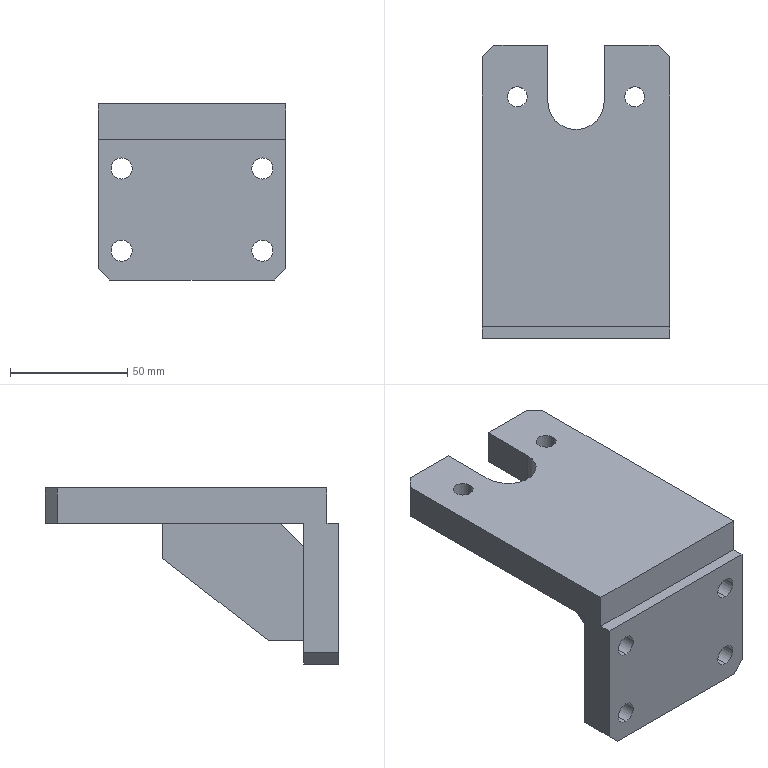Part | STEP file | YCD14007A-08.02.09-Horizontal Cylinder Connecting Plate-A3 | 1 solid | 36 faces | box 80 x 125 x 75 mm | volume 230135 mm3 | plane 23 | cylinder 13 | commonest cylinder face diameters 9 x8 8.5 x4 24 x1